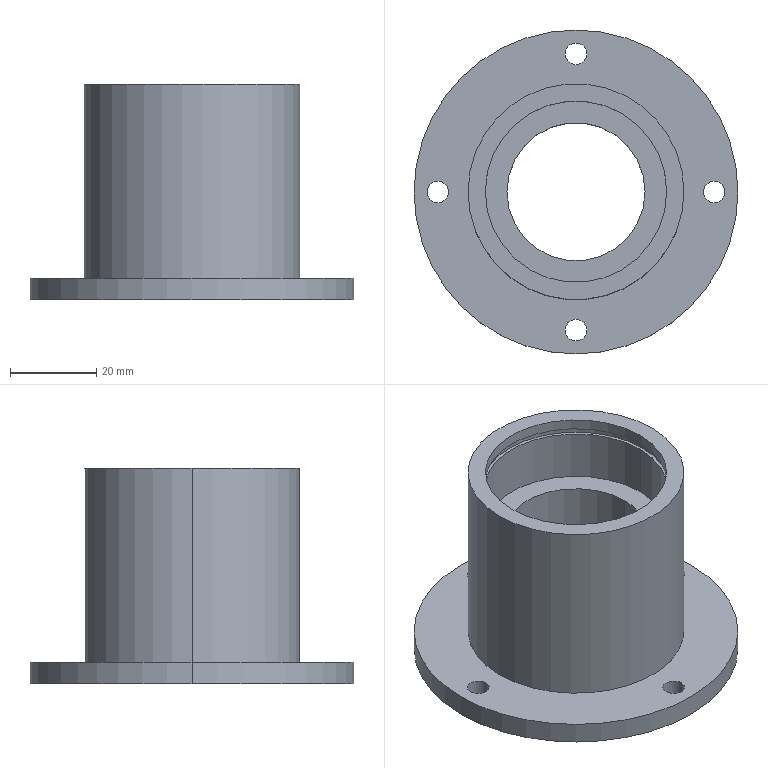Part | STEP file | Push-film drive bearing seat SGN-3-02 | 1 solid | 41 faces | box 75 x 75 x 50 mm | volume 49942 mm3 | cylinder 30 | plane 11 | commonest cylinder face diameters 5 x8 42 x8 43.5 x4 32 x2 47.35 x2 50 x2